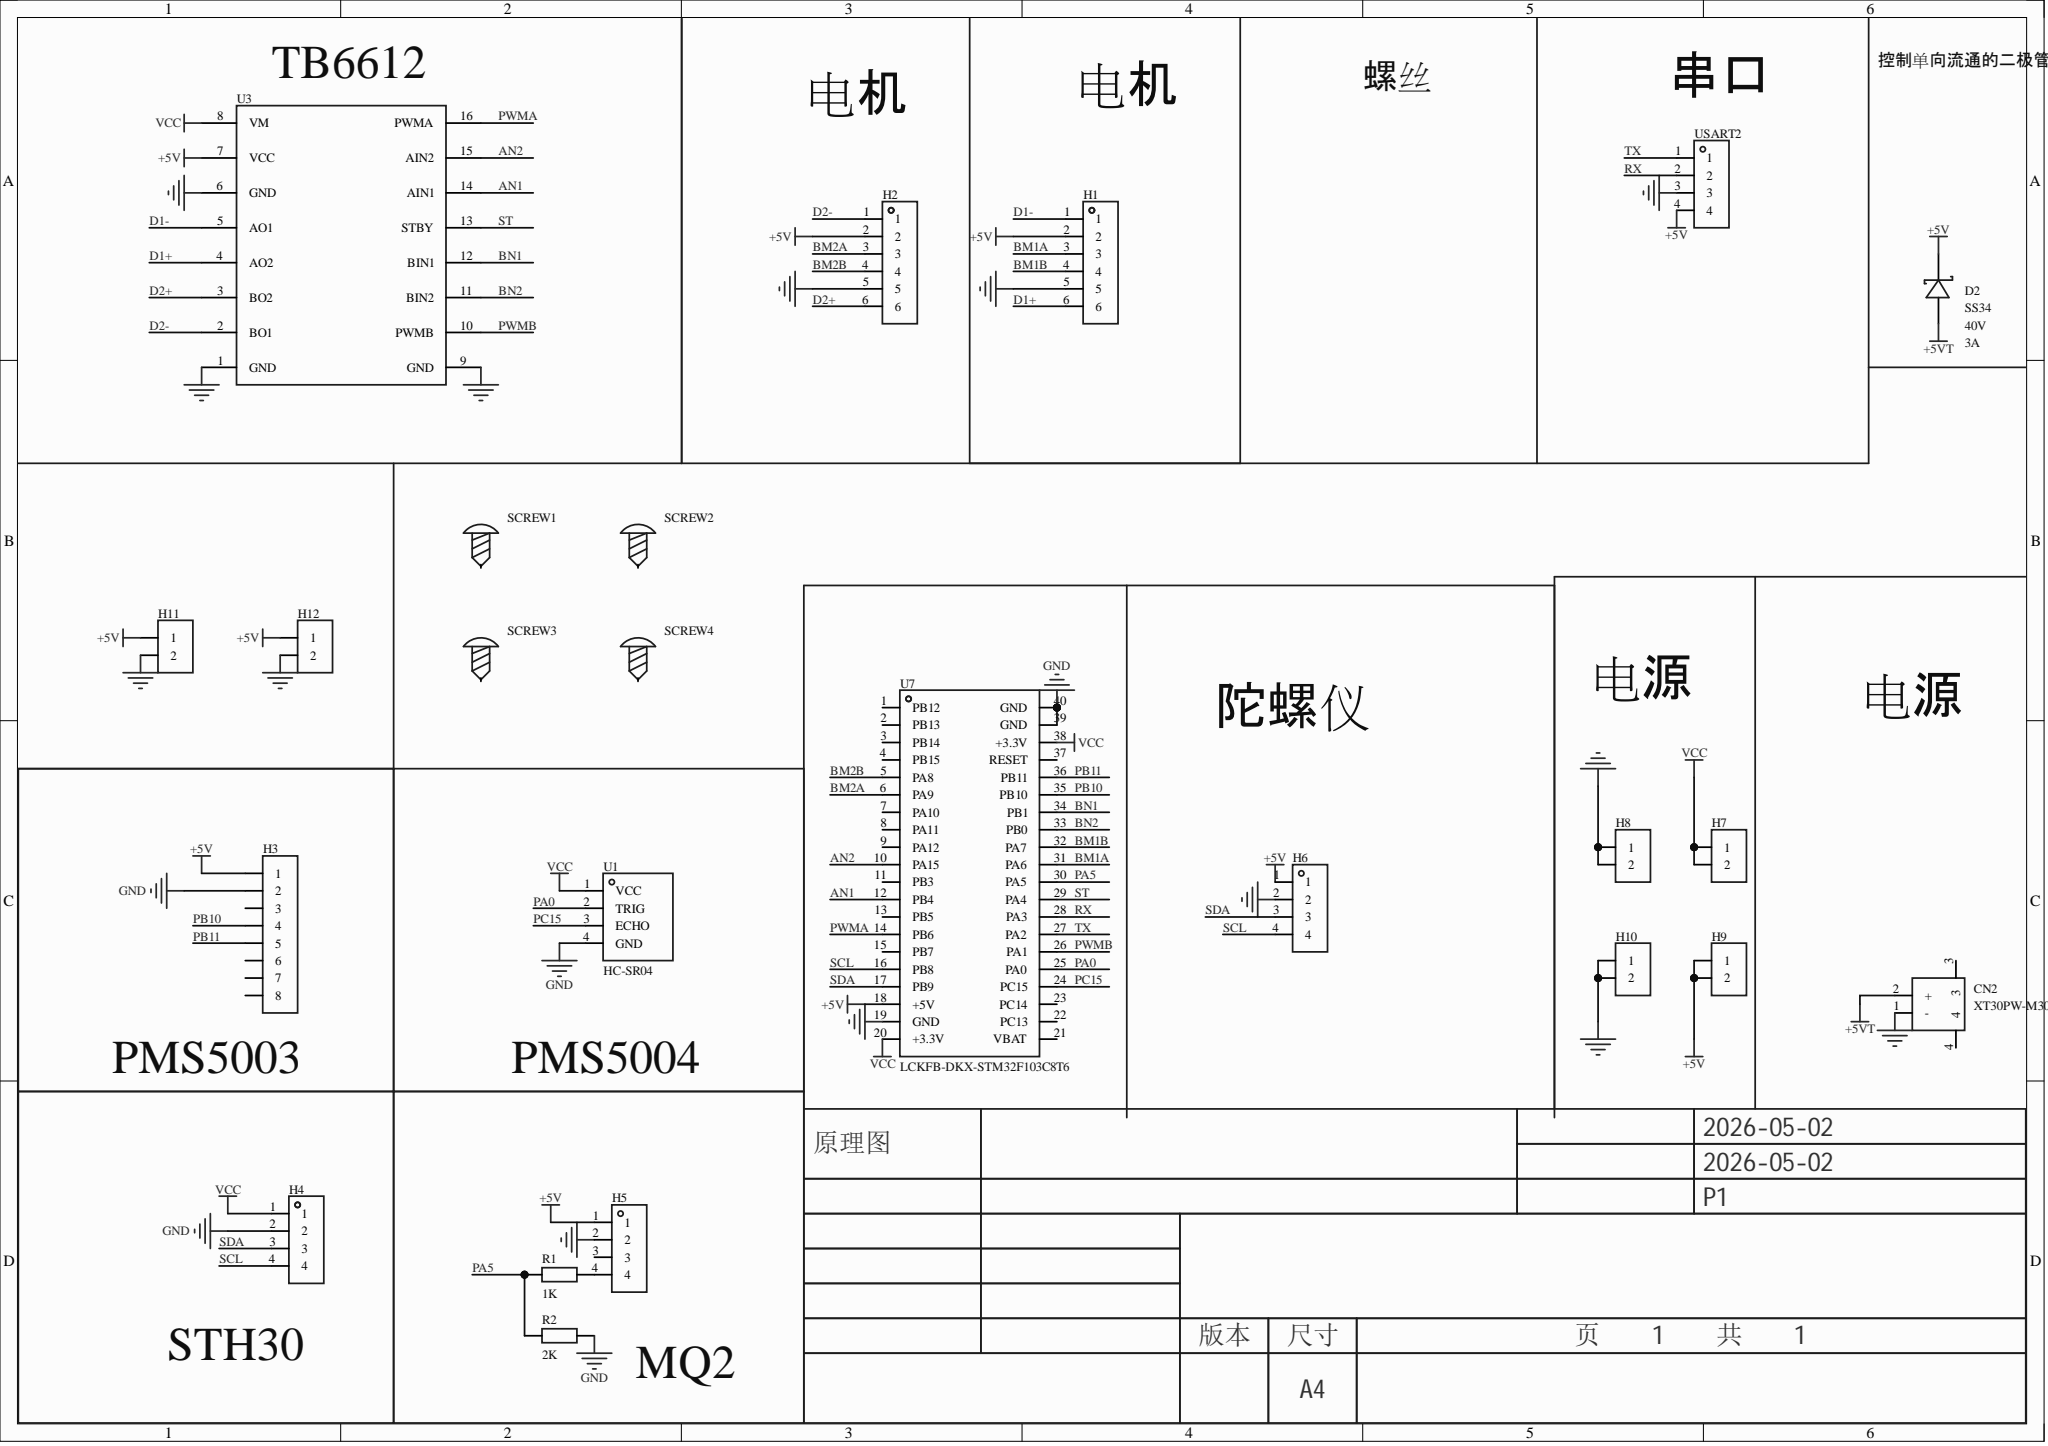Circuit board | Altium Designer | 24 parts | 29 nets
Bill of materials:
Comment,Description,Designator,Footprint,LibRef,Quantity
"XT30PW-M30.G.Y","","CN2","CONN-TH_XT30PW-M","XT30PW-M30.G.Y","1"
"SS34","","D2","SMC_L6.9-W5.9-LS7.9-RD","SS34_C154551","1"
"","","H1, H2","HDR-TH_6P-P2.54-V-F","HDR-F_2.54_1x6P","2"
"","","H3","HDR-TH_8P-P2.54-V-F-1","HDR-F_2.54_1x8P","1"
"","","H4","HDR-TH_4P-P2.54-V-F","HDR-F_2.54_1x4P","1"
"","","H5, H6, USART2","HDR-TH_4P-P2.54-V-M","HDR-M_2.54_1x4P","3"
"","","H7, H8, H9, H10, H11, H12","HDR-TH_2P-P2.54-V-F","HDR-F_2.54_1x2P","6"
"1K","","R1","R0603","Res_0603","1"
"2K","","R2","R0603","Res_0603","1"
"","","SCREW1, SCREW2, SCREW3, SCREW4","M2螺丝","M2螺丝","4"
"HC-SR04","","U1","TH_HC-SR04V","HC-SR04","1"
"","","U3","TB6612","TB6612","1"
"LCKFB-DKX-STM32F103C8T6","","U7","CONN-TH_L53.3-W22.9_STM32F103C8T6-CARD","LCKFB-DKX-STM32F103C8T6","1"
Netlist (Protel format):
[
CN2
CONN-TH_XT30PW-M
XT30PW-M30.G.Y



]
[
D2
SMC_L6.9-W5.9-LS7.9-RD
SS34



]
[
H1
HDR-TH_6P-P2.54-V-F




]
[
H2
HDR-TH_6P-P2.54-V-F




]
[
H3
HDR-TH_8P-P2.54-V-F-1




]
[
H4
HDR-TH_4P-P2.54-V-F




]
[
H5
HDR-TH_4P-P2.54-V-M




]
[
H6
HDR-TH_4P-P2.54-V-M




]
[
H7
HDR-TH_2P-P2.54-V-F




]
[
H8
HDR-TH_2P-P2.54-V-F




]
[
H9
HDR-TH_2P-P2.54-V-F




]
[
H10
HDR-TH_2P-P2.54-V-F




]
[
H11
HDR-TH_2P-P2.54-V-F




]
[
H12
HDR-TH_2P-P2.54-V-F




]
[
R1
R0603
1K



]
[
R2
R0603
2K



]
[
SCREW1
M2螺丝




]
[
SCREW2
M2螺丝




]
[
SCREW3
M2螺丝




]
[
SCREW4
M2螺丝




]
[
U1
TH_HC-SR04V
HC-SR04



]
[
U3
TB6612




]
[
U7
CONN-TH_L53.3-W22.9_STM32F103C8T6-CARD
LCKFB-DKX-STM32F103C8T6



]
[
USART2
HDR-TH_4P-P2.54-V-M




]
(
VCC
H4-1
H7-1
H7-2
U1-1
U3-8
U7-20
U7-38
)
(
TX
U7-27
USART2-1
)
(
ST
U3-13
U7-29
)
(
SDA
H4-3
H6-3
U7-17
)
(
SCL
H4-4
H6-4
U7-16
)
(
RX
U7-28
USART2-2
)
(
PWMB
U3-10
U7-26
)
(
PWMA
U3-16
U7-14
)
(
PC15
U1-3
U7-24
)
(
PB11
H3-5
U7-36
)
(
PB10
H3-4
U7-35
)
(
PA5
R1-1
R2-1
U7-30
)
(
PA0
U1-2
U7-25
)
(
NetH5_4
H5-4
R1-2
)
(
GND
CN2-1
H1-5
H2-5
H3-2
H4-2
H5-2
H6-2
H8-1
H8-2
H10-1
H10-2
H11-2
H12-2
R2-2
U1-4
U3-1
U3-6
U3-9
U7-19
U7-39
U7-40
USART2-3
)
(
D2-
H2-1
U3-2
)
(
D2+
H2-6
U3-3
)
(
D1-
H1-1
U3-5
)
(
D1+
H1-6
U3-4
)
(
BN2
U3-11
U7-33
)
(
BN1
U3-12
U7-34
)
(
BM2B
H2-4
U7-5
)
(
BM2A
H2-3
U7-6
)
(
BM1B
H1-4
U7-32
)
(
BM1A
H1-3
U7-31
)
(
AN2
U3-15
U7-10
)
(
AN1
U3-14
U7-12
)
(
+5VT
CN2-2
D2-2
)
(
+5V
D2-1
H1-2
H2-2
H3-1
H5-1
H6-1
H9-1
H9-2
H11-1
H12-1
U3-7
U7-18
USART2-4
)